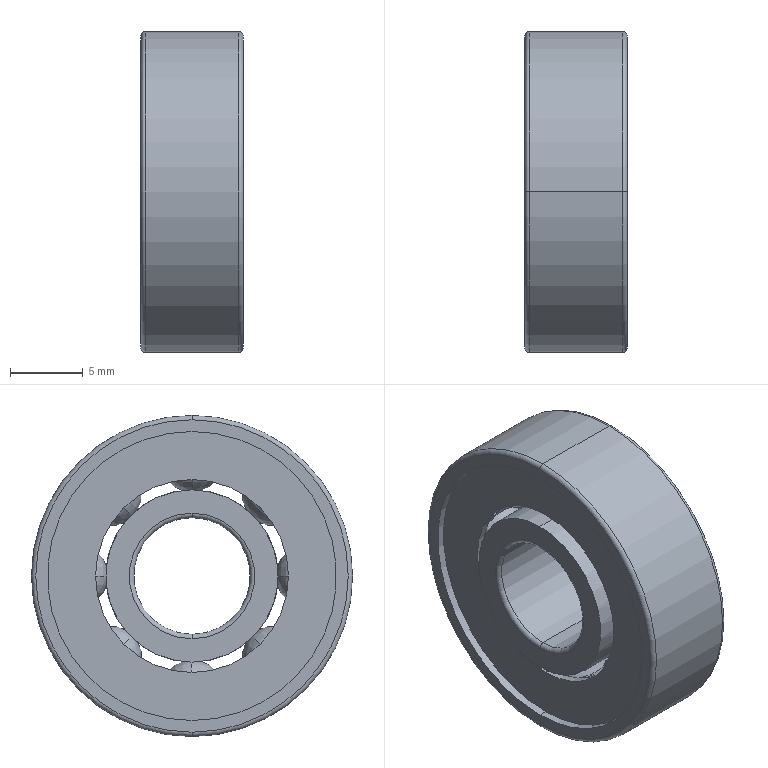Part | STEP file | GB/T 276-94 deep groove ball bearing 608-2Z | 1 solid | 144 faces | box 7 x 22 x 22 mm | volume 1460 mm3 | sphere 64 | torus 32 | cylinder 24 | plane 24 | commonest cylinder face diameters 19.8 x8 11.8 x4 13.219 x4 8 x2 14.617 x2 16.983 x2